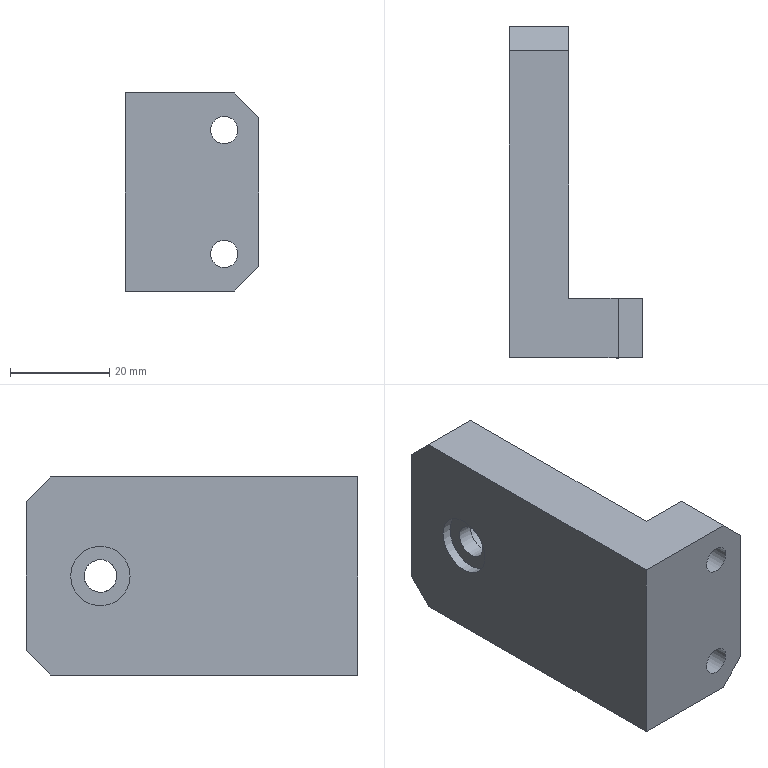Part | NX | 1 solid | 19 faces | box 27 x 67 x 40 mm | volume 37208 mm3 | plane 14 | cylinder 5 | commonest cylinder face diameters 5.5 x2 6.6 x1 11 x1 12 x1
STEP:
#1=CARTESIAN_POINT('',(-6.8,40.,-3.3));
#2=VERTEX_POINT('',#1);
#3=CARTESIAN_POINT('',(-6.8,40.,0.));
#4=DIRECTION('',(1.,0.,0.));
#5=DIRECTION('',(0.,0.,-1.));
#6=AXIS2_PLACEMENT_3D('',#3,#4,#5);
#7=CIRCLE('',#6,3.3);
#8=EDGE_CURVE('',#2,#2,#7,.T.);
#9=ORIENTED_EDGE('',*,*,#8,.T.);
#10=EDGE_LOOP('',(#9));
#11=FACE_BOUND('',#10,.T.);
#12=CARTESIAN_POINT('',(-10.,36.7,0.));
#13=VERTEX_POINT('',#12);
#14=CARTESIAN_POINT('',(-10.,40.,0.));
#15=DIRECTION('',(-1.,0.,0.));
#16=DIRECTION('',(0.,-1.,0.));
#17=AXIS2_PLACEMENT_3D('',#14,#15,#16);
#18=CIRCLE('',#17,3.3);
#19=EDGE_CURVE('',#13,#13,#18,.F.);
#20=ORIENTED_EDGE('',*,*,#19,.F.);
#21=EDGE_LOOP('',(#20));
#22=FACE_BOUND('',#21,.T.);
#23=CARTESIAN_POINT('',(0.,40.,0.));
#24=DIRECTION('',(1.,0.,0.));
#25=DIRECTION('',(0.,0.,-1.));
#26=AXIS2_PLACEMENT_3D('',#23,#24,#25);
#27=CYLINDRICAL_SURFACE('',#26,3.3);
#28=ADVANCED_FACE('',(#11,#22),#27,.F.);
#29=CARTESIAN_POINT('',(8.,-12.,-9.75));
#30=VERTEX_POINT('',#29);
#31=CARTESIAN_POINT('',(8.,-12.,-12.5));
#32=DIRECTION('',(0.,1.,0.));
#33=DIRECTION('',(0.,0.,1.));
#34=AXIS2_PLACEMENT_3D('',#31,#32,#33);
#35=CIRCLE('',#34,2.75);
#36=EDGE_CURVE('',#30,#30,#35,.T.);
#37=ORIENTED_EDGE('',*,*,#36,.T.);
#38=EDGE_LOOP('',(#37));
#39=FACE_BOUND('',#38,.T.);
#40=CARTESIAN_POINT('',(8.,-12.,15.25));
#41=VERTEX_POINT('',#40);
#42=CARTESIAN_POINT('',(8.,-12.,12.5));
#43=DIRECTION('',(0.,1.,0.));
#44=DIRECTION('',(0.,0.,1.));
#45=AXIS2_PLACEMENT_3D('',#42,#43,#44);
#46=CIRCLE('',#45,2.75);
#47=EDGE_CURVE('',#41,#41,#46,.T.);
#48=ORIENTED_EDGE('',*,*,#47,.T.);
#49=EDGE_LOOP('',(#48));
#50=FACE_BOUND('',#49,.T.);
#51=CARTESIAN_POINT('',(-12.,-12.,-20.));
#52=VERTEX_POINT('',#51);
#53=CARTESIAN_POINT('',(10.,-12.,-20.));
#54=VERTEX_POINT('',#53);
#55=CARTESIAN_POINT('',(0.,-12.,-20.));
#56=DIRECTION('',(1.,0.,0.));
#57=VECTOR('',#56,1000.);
#58=LINE('',#55,#57);
#59=EDGE_CURVE('',#52,#54,#58,.T.);
#60=ORIENTED_EDGE('',*,*,#59,.T.);
#61=CARTESIAN_POINT('',(15.,-12.,-15.));
#62=VERTEX_POINT('',#61);
#63=CARTESIAN_POINT('',(10.,-12.,-20.));
#64=DIRECTION('',(-0.7071,0.,-0.7071));
#65=VECTOR('',#64,1000.);
#66=LINE('',#63,#65);
#67=EDGE_CURVE('',#54,#62,#66,.F.);
#68=ORIENTED_EDGE('',*,*,#67,.T.);
#69=CARTESIAN_POINT('',(15.,-12.,15.));
#70=VERTEX_POINT('',#69);
#71=CARTESIAN_POINT('',(15.,-12.,20.));
#72=DIRECTION('',(0.,0.,-1.));
#73=VECTOR('',#72,1000.);
#74=LINE('',#71,#73);
#75=EDGE_CURVE('',#70,#62,#74,.T.);
#76=ORIENTED_EDGE('',*,*,#75,.F.);
#77=CARTESIAN_POINT('',(10.,-12.,20.));
#78=VERTEX_POINT('',#77);
#79=CARTESIAN_POINT('',(15.,-12.,15.));
#80=DIRECTION('',(-0.7071,0.,0.7071));
#81=VECTOR('',#80,1000.);
#82=LINE('',#79,#81);
#83=EDGE_CURVE('',#70,#78,#82,.T.);
#84=ORIENTED_EDGE('',*,*,#83,.T.);
#85=CARTESIAN_POINT('',(-12.,-12.,20.));
#86=VERTEX_POINT('',#85);
#87=CARTESIAN_POINT('',(0.,-12.,20.));
#88=DIRECTION('',(1.,0.,0.));
#89=VECTOR('',#88,1000.);
#90=LINE('',#87,#89);
#91=EDGE_CURVE('',#86,#78,#90,.T.);
#92=ORIENTED_EDGE('',*,*,#91,.F.);
#93=CARTESIAN_POINT('',(-12.,-12.,20.));
#94=DIRECTION('',(0.,0.,-1.));
#95=VECTOR('',#94,1000.);
#96=LINE('',#93,#95);
#97=EDGE_CURVE('',#86,#52,#96,.T.);
#98=ORIENTED_EDGE('',*,*,#97,.T.);
#99=EDGE_LOOP('',(#60,#68,#76,#84,#92,#98));
#100=FACE_BOUND('',#99,.T.);
#101=CARTESIAN_POINT('',(0.,-12.,20.));
#102=DIRECTION('',(0.,1.,0.));
#103=DIRECTION('',(0.,0.,1.));
#104=AXIS2_PLACEMENT_3D('',#101,#102,#103);
#105=PLANE('',#104);
#106=ADVANCED_FACE('',(#39,#50,#100),#105,.F.);
#107=ORIENTED_EDGE('',*,*,#75,.T.);
#108=CARTESIAN_POINT('',(15.,0.,-15.));
#109=VERTEX_POINT('',#108);
#110=CARTESIAN_POINT('',(15.,0.,-15.));
#111=DIRECTION('',(0.,1.,0.));
#112=VECTOR('',#111,1000.);
#113=LINE('',#110,#112);
#114=EDGE_CURVE('',#62,#109,#113,.T.);
#115=ORIENTED_EDGE('',*,*,#114,.T.);
#116=CARTESIAN_POINT('',(15.,0.,15.));
#117=VERTEX_POINT('',#116);
#118=CARTESIAN_POINT('',(15.,0.,20.));
#119=DIRECTION('',(0.,0.,-1.));
#120=VECTOR('',#119,1000.);
#121=LINE('',#118,#120);
#122=EDGE_CURVE('',#117,#109,#121,.T.);
#123=ORIENTED_EDGE('',*,*,#122,.F.);
#124=CARTESIAN_POINT('',(15.,-12.,15.));
#125=DIRECTION('',(0.,-1.,0.));
#126=VECTOR('',#125,1000.);
#127=LINE('',#124,#126);
#128=EDGE_CURVE('',#117,#70,#127,.T.);
#129=ORIENTED_EDGE('',*,*,#128,.T.);
#130=EDGE_LOOP('',(#107,#115,#123,#129));
#131=FACE_BOUND('',#130,.T.);
#132=CARTESIAN_POINT('',(15.,0.,20.));
#133=DIRECTION('',(1.,0.,0.));
#134=DIRECTION('',(0.,0.,-1.));
#135=AXIS2_PLACEMENT_3D('',#132,#133,#134);
#136=PLANE('',#135);
#137=ADVANCED_FACE('',(#131),#136,.T.);
#138=CARTESIAN_POINT('',(8.,0.,-9.75));
#139=VERTEX_POINT('',#138);
#140=CARTESIAN_POINT('',(8.,0.,-12.5));
#141=DIRECTION('',(0.,1.,0.));
#142=DIRECTION('',(0.,0.,1.));
#143=AXIS2_PLACEMENT_3D('',#140,#141,#142);
#144=CIRCLE('',#143,2.75);
#145=EDGE_CURVE('',#139,#139,#144,.T.);
#146=ORIENTED_EDGE('',*,*,#145,.F.);
#147=EDGE_LOOP('',(#146));
#148=FACE_BOUND('',#147,.T.);
#149=CARTESIAN_POINT('',(8.,0.,15.25));
#150=VERTEX_POINT('',#149);
#151=CARTESIAN_POINT('',(8.,0.,12.5));
#152=DIRECTION('',(0.,1.,0.));
#153=DIRECTION('',(0.,0.,1.));
#154=AXIS2_PLACEMENT_3D('',#151,#152,#153);
#155=CIRCLE('',#154,2.75);
#156=EDGE_CURVE('',#150,#150,#155,.T.);
#157=ORIENTED_EDGE('',*,*,#156,.F.);
#158=EDGE_LOOP('',(#157));
#159=FACE_BOUND('',#158,.T.);
#160=ORIENTED_EDGE('',*,*,#122,.T.);
#161=CARTESIAN_POINT('',(10.,0.,-20.));
#162=VERTEX_POINT('',#161);
#163=CARTESIAN_POINT('',(25.,0.,-5.));
#164=DIRECTION('',(0.7071,0.,0.7071));
#165=VECTOR('',#164,1000.);
#166=LINE('',#163,#165);
#167=EDGE_CURVE('',#109,#162,#166,.F.);
#168=ORIENTED_EDGE('',*,*,#167,.T.);
#169=CARTESIAN_POINT('',(0.,0.,-20.));
#170=VERTEX_POINT('',#169);
#171=CARTESIAN_POINT('',(0.,0.,-20.));
#172=DIRECTION('',(1.,0.,0.));
#173=VECTOR('',#172,1000.);
#174=LINE('',#171,#173);
#175=EDGE_CURVE('',#170,#162,#174,.T.);
#176=ORIENTED_EDGE('',*,*,#175,.F.);
#177=CARTESIAN_POINT('',(0.,0.,20.));
#178=VERTEX_POINT('',#177);
#179=CARTESIAN_POINT('',(0.,0.,20.));
#180=DIRECTION('',(0.,0.,-1.));
#181=VECTOR('',#180,1000.);
#182=LINE('',#179,#181);
#183=EDGE_CURVE('',#178,#170,#182,.T.);
#184=ORIENTED_EDGE('',*,*,#183,.F.);
#185=CARTESIAN_POINT('',(10.,0.,20.));
#186=VERTEX_POINT('',#185);
#187=CARTESIAN_POINT('',(0.,0.,20.));
#188=DIRECTION('',(1.,0.,0.));
#189=VECTOR('',#188,1000.);
#190=LINE('',#187,#189);
#191=EDGE_CURVE('',#178,#186,#190,.T.);
#192=ORIENTED_EDGE('',*,*,#191,.T.);
#193=CARTESIAN_POINT('',(5.,0.,25.));
#194=DIRECTION('',(0.7071,0.,-0.7071));
#195=VECTOR('',#194,1000.);
#196=LINE('',#193,#195);
#197=EDGE_CURVE('',#186,#117,#196,.T.);
#198=ORIENTED_EDGE('',*,*,#197,.T.);
#199=EDGE_LOOP('',(#160,#168,#176,#184,#192,#198));
#200=FACE_BOUND('',#199,.T.);
#201=CARTESIAN_POINT('',(0.,0.,20.));
#202=DIRECTION('',(0.,1.,0.));
#203=DIRECTION('',(0.,0.,1.));
#204=AXIS2_PLACEMENT_3D('',#201,#202,#203);
#205=PLANE('',#204);
#206=ADVANCED_FACE('',(#148,#159,#200),#205,.T.);
#207=CARTESIAN_POINT('',(0.,40.,-5.5));
#208=VERTEX_POINT('',#207);
#209=CARTESIAN_POINT('',(0.,40.,0.));
#210=DIRECTION('',(1.,0.,0.));
#211=DIRECTION('',(0.,0.,-1.));
#212=AXIS2_PLACEMENT_3D('',#209,#210,#211);
#213=CIRCLE('',#212,5.5);
#214=EDGE_CURVE('',#208,#208,#213,.T.);
#215=ORIENTED_EDGE('',*,*,#214,.F.);
#216=EDGE_LOOP('',(#215));
#217=FACE_BOUND('',#216,.T.);
#218=CARTESIAN_POINT('',(0.,50.,-20.));
#219=VERTEX_POINT('',#218);
#220=CARTESIAN_POINT('',(0.,55.,-20.));
#221=DIRECTION('',(0.,-1.,0.));
#222=VECTOR('',#221,1000.);
#223=LINE('',#220,#222);
#224=EDGE_CURVE('',#219,#170,#223,.T.);
#225=ORIENTED_EDGE('',*,*,#224,.F.);
#226=CARTESIAN_POINT('',(0.,55.,-15.));
#227=VERTEX_POINT('',#226);
#228=CARTESIAN_POINT('',(0.,72.5,2.5));
#229=DIRECTION('',(0.,-0.7071,-0.7071));
#230=VECTOR('',#229,1000.);
#231=LINE('',#228,#230);
#232=EDGE_CURVE('',#219,#227,#231,.F.);
#233=ORIENTED_EDGE('',*,*,#232,.T.);
#234=CARTESIAN_POINT('',(0.,55.,15.));
#235=VERTEX_POINT('',#234);
#236=CARTESIAN_POINT('',(0.,55.,20.));
#237=DIRECTION('',(0.,0.,-1.));
#238=VECTOR('',#237,1000.);
#239=LINE('',#236,#238);
#240=EDGE_CURVE('',#235,#227,#239,.T.);
#241=ORIENTED_EDGE('',*,*,#240,.F.);
#242=CARTESIAN_POINT('',(0.,50.,20.));
#243=VERTEX_POINT('',#242);
#244=CARTESIAN_POINT('',(0.,52.5,17.5));
#245=DIRECTION('',(0.,-0.7071,0.7071));
#246=VECTOR('',#245,1000.);
#247=LINE('',#244,#246);
#248=EDGE_CURVE('',#235,#243,#247,.T.);
#249=ORIENTED_EDGE('',*,*,#248,.T.);
#250=CARTESIAN_POINT('',(0.,55.,20.));
#251=DIRECTION('',(0.,-1.,0.));
#252=VECTOR('',#251,1000.);
#253=LINE('',#250,#252);
#254=EDGE_CURVE('',#243,#178,#253,.T.);
#255=ORIENTED_EDGE('',*,*,#254,.T.);
#256=ORIENTED_EDGE('',*,*,#183,.T.);
#257=EDGE_LOOP('',(#225,#233,#241,#249,#255,#256));
#258=FACE_BOUND('',#257,.T.);
#259=CARTESIAN_POINT('',(0.,55.,20.));
#260=DIRECTION('',(1.,0.,0.));
#261=DIRECTION('',(0.,1.,0.));
#262=AXIS2_PLACEMENT_3D('',#259,#260,#261);
#263=PLANE('',#262);
#264=ADVANCED_FACE('',(#217,#258),#263,.T.);
#265=ORIENTED_EDGE('',*,*,#240,.T.);
#266=CARTESIAN_POINT('',(-12.,55.,-15.));
#267=VERTEX_POINT('',#266);
#268=CARTESIAN_POINT('',(-12.,55.,-15.));
#269=DIRECTION('',(-1.,0.,0.));
#270=VECTOR('',#269,1000.);
#271=LINE('',#268,#270);
#272=EDGE_CURVE('',#227,#267,#271,.T.);
#273=ORIENTED_EDGE('',*,*,#272,.T.);
#274=CARTESIAN_POINT('',(-12.,55.,15.));
#275=VERTEX_POINT('',#274);
#276=CARTESIAN_POINT('',(-12.,55.,20.));
#277=DIRECTION('',(0.,0.,-1.));
#278=VECTOR('',#277,1000.);
#279=LINE('',#276,#278);
#280=EDGE_CURVE('',#275,#267,#279,.T.);
#281=ORIENTED_EDGE('',*,*,#280,.F.);
#282=CARTESIAN_POINT('',(0.,55.,15.));
#283=DIRECTION('',(1.,0.,0.));
#284=VECTOR('',#283,1000.);
#285=LINE('',#282,#284);
#286=EDGE_CURVE('',#275,#235,#285,.T.);
#287=ORIENTED_EDGE('',*,*,#286,.T.);
#288=EDGE_LOOP('',(#265,#273,#281,#287));
#289=FACE_BOUND('',#288,.T.);
#290=CARTESIAN_POINT('',(-12.,55.,20.));
#291=DIRECTION('',(0.,1.,0.));
#292=DIRECTION('',(0.,0.,1.));
#293=AXIS2_PLACEMENT_3D('',#290,#291,#292);
#294=PLANE('',#293);
#295=ADVANCED_FACE('',(#289),#294,.T.);
#296=CARTESIAN_POINT('',(-12.,34.,0.));
#297=VERTEX_POINT('',#296);
#298=CARTESIAN_POINT('',(-12.,40.,0.));
#299=DIRECTION('',(-1.,0.,0.));
#300=DIRECTION('',(0.,-1.,0.));
#301=AXIS2_PLACEMENT_3D('',#298,#299,#300);
#302=CIRCLE('',#301,6.);
#303=EDGE_CURVE('',#297,#297,#302,.T.);
#304=ORIENTED_EDGE('',*,*,#303,.F.);
#305=EDGE_LOOP('',(#304));
#306=FACE_BOUND('',#305,.T.);
#307=ORIENTED_EDGE('',*,*,#280,.T.);
#308=CARTESIAN_POINT('',(-12.,50.,-20.));
#309=VERTEX_POINT('',#308);
#310=CARTESIAN_POINT('',(-12.,50.,-20.));
#311=DIRECTION('',(0.,0.7071,0.7071));
#312=VECTOR('',#311,1000.);
#313=LINE('',#310,#312);
#314=EDGE_CURVE('',#267,#309,#313,.F.);
#315=ORIENTED_EDGE('',*,*,#314,.T.);
#316=CARTESIAN_POINT('',(-12.,55.,-20.));
#317=DIRECTION('',(0.,-1.,0.));
#318=VECTOR('',#317,1000.);
#319=LINE('',#316,#318);
#320=EDGE_CURVE('',#309,#52,#319,.T.);
#321=ORIENTED_EDGE('',*,*,#320,.T.);
#322=ORIENTED_EDGE('',*,*,#97,.F.);
#323=CARTESIAN_POINT('',(-12.,50.,20.));
#324=VERTEX_POINT('',#323);
#325=CARTESIAN_POINT('',(-12.,55.,20.));
#326=DIRECTION('',(0.,-1.,0.));
#327=VECTOR('',#326,1000.);
#328=LINE('',#325,#327);
#329=EDGE_CURVE('',#324,#86,#328,.T.);
#330=ORIENTED_EDGE('',*,*,#329,.F.);
#331=CARTESIAN_POINT('',(-12.,55.,15.));
#332=DIRECTION('',(0.,0.7071,-0.7071));
#333=VECTOR('',#332,1000.);
#334=LINE('',#331,#333);
#335=EDGE_CURVE('',#324,#275,#334,.T.);
#336=ORIENTED_EDGE('',*,*,#335,.T.);
#337=EDGE_LOOP('',(#307,#315,#321,#322,#330,#336));
#338=FACE_BOUND('',#337,.T.);
#339=CARTESIAN_POINT('',(-12.,55.,20.));
#340=DIRECTION('',(1.,0.,0.));
#341=DIRECTION('',(0.,1.,0.));
#342=AXIS2_PLACEMENT_3D('',#339,#340,#341);
#343=PLANE('',#342);
#344=ADVANCED_FACE('',(#306,#338),#343,.F.);
#345=ORIENTED_EDGE('',*,*,#254,.F.);
#346=CARTESIAN_POINT('',(-12.,50.,20.));
#347=DIRECTION('',(-1.,0.,0.));
#348=VECTOR('',#347,1000.);
#349=LINE('',#346,#348);
#350=EDGE_CURVE('',#243,#324,#349,.T.);
#351=ORIENTED_EDGE('',*,*,#350,.T.);
#352=ORIENTED_EDGE('',*,*,#329,.T.);
#353=ORIENTED_EDGE('',*,*,#91,.T.);
#354=CARTESIAN_POINT('',(10.,0.,20.));
#355=DIRECTION('',(0.,1.,0.));
#356=VECTOR('',#355,1000.);
#357=LINE('',#354,#356);
#358=EDGE_CURVE('',#78,#186,#357,.T.);
#359=ORIENTED_EDGE('',*,*,#358,.T.);
#360=ORIENTED_EDGE('',*,*,#191,.F.);
#361=EDGE_LOOP('',(#345,#351,#352,#353,#359,#360));
#362=FACE_BOUND('',#361,.T.);
#363=CARTESIAN_POINT('',(0.,0.,20.));
#364=DIRECTION('',(0.,0.,-1.));
#365=DIRECTION('',(-1.,0.,0.));
#366=AXIS2_PLACEMENT_3D('',#363,#364,#365);
#367=PLANE('',#366);
#368=ADVANCED_FACE('',(#362),#367,.F.);
#369=ORIENTED_EDGE('',*,*,#320,.F.);
#370=CARTESIAN_POINT('',(0.,50.,-20.));
#371=DIRECTION('',(1.,0.,0.));
#372=VECTOR('',#371,1000.);
#373=LINE('',#370,#372);
#374=EDGE_CURVE('',#309,#219,#373,.T.);
#375=ORIENTED_EDGE('',*,*,#374,.T.);
#376=ORIENTED_EDGE('',*,*,#224,.T.);
#377=ORIENTED_EDGE('',*,*,#175,.T.);
#378=CARTESIAN_POINT('',(10.,0.,-20.));
#379=DIRECTION('',(0.,-1.,0.));
#380=VECTOR('',#379,1000.);
#381=LINE('',#378,#380);
#382=EDGE_CURVE('',#162,#54,#381,.T.);
#383=ORIENTED_EDGE('',*,*,#382,.T.);
#384=ORIENTED_EDGE('',*,*,#59,.F.);
#385=EDGE_LOOP('',(#369,#375,#376,#377,#383,#384));
#386=FACE_BOUND('',#385,.T.);
#387=CARTESIAN_POINT('',(0.,0.,-20.));
#388=DIRECTION('',(0.,0.,-1.));
#389=DIRECTION('',(-1.,0.,0.));
#390=AXIS2_PLACEMENT_3D('',#387,#388,#389);
#391=PLANE('',#390);
#392=ADVANCED_FACE('',(#386),#391,.T.);
#393=ORIENTED_EDGE('',*,*,#314,.F.);
#394=ORIENTED_EDGE('',*,*,#272,.F.);
#395=ORIENTED_EDGE('',*,*,#232,.F.);
#396=ORIENTED_EDGE('',*,*,#374,.F.);
#397=EDGE_LOOP('',(#393,#394,#395,#396));
#398=FACE_BOUND('',#397,.T.);
#399=CARTESIAN_POINT('',(0.,50.,-20.));
#400=DIRECTION('',(0.,-0.7071,0.7071));
#401=DIRECTION('',(1.,0.,0.));
#402=AXIS2_PLACEMENT_3D('',#399,#400,#401);
#403=PLANE('',#402);
#404=ADVANCED_FACE('',(#398),#403,.F.);
#405=ORIENTED_EDGE('',*,*,#335,.F.);
#406=ORIENTED_EDGE('',*,*,#350,.F.);
#407=ORIENTED_EDGE('',*,*,#248,.F.);
#408=ORIENTED_EDGE('',*,*,#286,.F.);
#409=EDGE_LOOP('',(#405,#406,#407,#408));
#410=FACE_BOUND('',#409,.T.);
#411=CARTESIAN_POINT('',(-12.,55.,15.));
#412=DIRECTION('',(0.,0.7071,0.7071));
#413=DIRECTION('',(-1.,0.,0.));
#414=AXIS2_PLACEMENT_3D('',#411,#412,#413);
#415=PLANE('',#414);
#416=ADVANCED_FACE('',(#410),#415,.T.);
#417=ORIENTED_EDGE('',*,*,#167,.F.);
#418=ORIENTED_EDGE('',*,*,#114,.F.);
#419=ORIENTED_EDGE('',*,*,#67,.F.);
#420=ORIENTED_EDGE('',*,*,#382,.F.);
#421=EDGE_LOOP('',(#417,#418,#419,#420));
#422=FACE_BOUND('',#421,.T.);
#423=CARTESIAN_POINT('',(10.,0.,-20.));
#424=DIRECTION('',(-0.7071,0.,0.7071));
#425=DIRECTION('',(0.,-1.,0.));
#426=AXIS2_PLACEMENT_3D('',#423,#424,#425);
#427=PLANE('',#426);
#428=ADVANCED_FACE('',(#422),#427,.F.);
#429=ORIENTED_EDGE('',*,*,#197,.F.);
#430=ORIENTED_EDGE('',*,*,#358,.F.);
#431=ORIENTED_EDGE('',*,*,#83,.F.);
#432=ORIENTED_EDGE('',*,*,#128,.F.);
#433=EDGE_LOOP('',(#429,#430,#431,#432));
#434=FACE_BOUND('',#433,.T.);
#435=CARTESIAN_POINT('',(15.,0.,15.));
#436=DIRECTION('',(0.7071,0.,0.7071));
#437=DIRECTION('',(0.,1.,0.));
#438=AXIS2_PLACEMENT_3D('',#435,#436,#437);
#439=PLANE('',#438);
#440=ADVANCED_FACE('',(#434),#439,.T.);
#441=ORIENTED_EDGE('',*,*,#47,.F.);
#442=EDGE_LOOP('',(#441));
#443=FACE_BOUND('',#442,.T.);
#444=ORIENTED_EDGE('',*,*,#156,.T.);
#445=EDGE_LOOP('',(#444));
#446=FACE_BOUND('',#445,.T.);
#447=CARTESIAN_POINT('',(8.,0.,12.5));
#448=DIRECTION('',(0.,1.,0.));
#449=DIRECTION('',(0.,0.,1.));
#450=AXIS2_PLACEMENT_3D('',#447,#448,#449);
#451=CYLINDRICAL_SURFACE('',#450,2.75);
#452=ADVANCED_FACE('',(#443,#446),#451,.F.);
#453=ORIENTED_EDGE('',*,*,#36,.F.);
#454=EDGE_LOOP('',(#453));
#455=FACE_BOUND('',#454,.T.);
#456=ORIENTED_EDGE('',*,*,#145,.T.);
#457=EDGE_LOOP('',(#456));
#458=FACE_BOUND('',#457,.T.);
#459=CARTESIAN_POINT('',(8.,0.,-12.5));
#460=DIRECTION('',(0.,1.,0.));
#461=DIRECTION('',(0.,0.,1.));
#462=AXIS2_PLACEMENT_3D('',#459,#460,#461);
#463=CYLINDRICAL_SURFACE('',#462,2.75);
#464=ADVANCED_FACE('',(#455,#458),#463,.F.);
#465=ORIENTED_EDGE('',*,*,#8,.F.);
#466=EDGE_LOOP('',(#465));
#467=FACE_BOUND('',#466,.T.);
#468=CARTESIAN_POINT('',(-6.8,40.,-5.5));
#469=VERTEX_POINT('',#468);
#470=CARTESIAN_POINT('',(-6.8,40.,0.));
#471=DIRECTION('',(1.,0.,0.));
#472=DIRECTION('',(0.,0.,-1.));
#473=AXIS2_PLACEMENT_3D('',#470,#471,#472);
#474=CIRCLE('',#473,5.5);
#475=EDGE_CURVE('',#469,#469,#474,.T.);
#476=ORIENTED_EDGE('',*,*,#475,.T.);
#477=EDGE_LOOP('',(#476));
#478=FACE_BOUND('',#477,.T.);
#479=CARTESIAN_POINT('',(-6.8,43.3,0.));
#480=DIRECTION('',(-1.,0.,0.));
#481=DIRECTION('',(0.,0.,1.));
#482=AXIS2_PLACEMENT_3D('',#479,#480,#481);
#483=PLANE('',#482);
#484=ADVANCED_FACE('',(#467,#478),#483,.F.);
#485=ORIENTED_EDGE('',*,*,#475,.F.);
#486=EDGE_LOOP('',(#485));
#487=FACE_BOUND('',#486,.T.);
#488=ORIENTED_EDGE('',*,*,#214,.T.);
#489=EDGE_LOOP('',(#488));
#490=FACE_BOUND('',#489,.T.);
#491=CARTESIAN_POINT('',(0.,40.,0.));
#492=DIRECTION('',(1.,0.,0.));
#493=DIRECTION('',(0.,0.,-1.));
#494=AXIS2_PLACEMENT_3D('',#491,#492,#493);
#495=CYLINDRICAL_SURFACE('',#494,5.5);
#496=ADVANCED_FACE('',(#487,#490),#495,.F.);
#497=CARTESIAN_POINT('',(-10.,34.,0.));
#498=VERTEX_POINT('',#497);
#499=CARTESIAN_POINT('',(-10.,40.,0.));
#500=DIRECTION('',(-1.,0.,0.));
#501=DIRECTION('',(0.,-1.,0.));
#502=AXIS2_PLACEMENT_3D('',#499,#500,#501);
#503=CIRCLE('',#502,6.);
#504=EDGE_CURVE('',#498,#498,#503,.T.);
#505=ORIENTED_EDGE('',*,*,#504,.T.);
#506=EDGE_LOOP('',(#505));
#507=FACE_BOUND('',#506,.T.);
#508=ORIENTED_EDGE('',*,*,#19,.T.);
#509=EDGE_LOOP('',(#508));
#510=FACE_BOUND('',#509,.T.);
#511=CARTESIAN_POINT('',(-10.,40.,0.));
#512=DIRECTION('',(-1.,0.,0.));
#513=DIRECTION('',(0.,-1.,0.));
#514=AXIS2_PLACEMENT_3D('',#511,#512,#513);
#515=PLANE('',#514);
#516=ADVANCED_FACE('',(#507,#510),#515,.T.);
#517=ORIENTED_EDGE('',*,*,#504,.F.);
#518=EDGE_LOOP('',(#517));
#519=FACE_BOUND('',#518,.T.);
#520=ORIENTED_EDGE('',*,*,#303,.T.);
#521=EDGE_LOOP('',(#520));
#522=FACE_BOUND('',#521,.T.);
#523=CARTESIAN_POINT('',(-10.,40.,0.));
#524=DIRECTION('',(-1.,0.,0.));
#525=DIRECTION('',(0.,-1.,0.));
#526=AXIS2_PLACEMENT_3D('',#523,#524,#525);
#527=CYLINDRICAL_SURFACE('',#526,6.);
#528=ADVANCED_FACE('',(#519,#522),#527,.F.);
#529=CLOSED_SHELL('',(#28,#106,#137,#206,#264,#295,#344,#368,#392,#404,#416,#428,#440,#452,#464,#484,#496,#516,#528));
#530=MANIFOLD_SOLID_BREP('',#529);
#531=(LENGTH_UNIT()NAMED_UNIT(*)SI_UNIT(.MILLI.,.METRE.));
#532=UNCERTAINTY_MEASURE_WITH_UNIT(LENGTH_MEASURE(0.00001),#531,'','');
#533=(NAMED_UNIT(*)PLANE_ANGLE_UNIT()SI_UNIT($,.RADIAN.));
#534=(NAMED_UNIT(*)SI_UNIT($,.STERADIAN.)SOLID_ANGLE_UNIT());
#535=(GEOMETRIC_REPRESENTATION_CONTEXT(3)GLOBAL_UNCERTAINTY_ASSIGNED_CONTEXT((#532))GLOBAL_UNIT_ASSIGNED_CONTEXT((#531,#533,#534))REPRESENTATION_CONTEXT('',''));
#536=ADVANCED_BREP_SHAPE_REPRESENTATION('',(#530),#535);